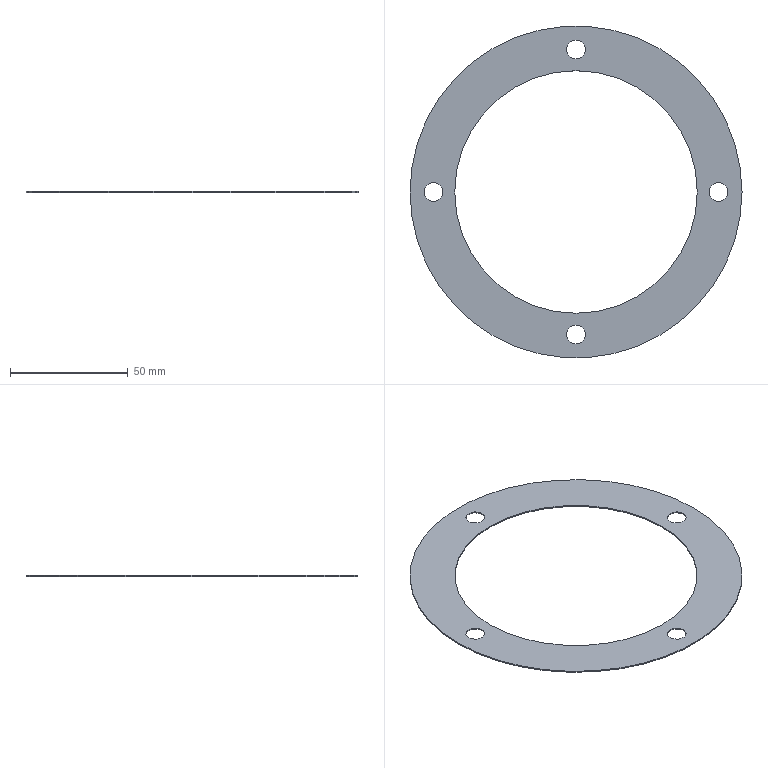Part | SolidWorks | features Extrusion 1, ICE 1 | 1 solid | 14 faces | box 141 x 141 x 0.5 mm | volume 3541 mm3 | cylinder 12 | plane 2 | commonest cylinder face diameters 8 x8 103 x2 141 x2
STEP:
#1=CARTESIAN_POINT('',(-64.5,0.,0.));
#2=VERTEX_POINT('',#1);
#3=CARTESIAN_POINT('',(-56.5,0.,0.));
#4=VERTEX_POINT('',#3);
#5=CARTESIAN_POINT('',(-60.5,0.,0.));
#6=DIRECTION('',(0.,0.,1.));
#7=DIRECTION('',(1.,0.,0.));
#8=AXIS2_PLACEMENT_3D('',#5,#6,#7);
#9=CIRCLE('',#8,4.);
#10=EDGE_CURVE('',#2,#4,#9,.T.);
#11=ORIENTED_EDGE('',*,*,#10,.F.);
#12=CARTESIAN_POINT('',(-64.5,0.,0.5));
#13=VERTEX_POINT('',#12);
#14=CARTESIAN_POINT('',(-64.5,0.,0.));
#15=DIRECTION('',(0.,0.,1.));
#16=VECTOR('',#15,1000.);
#17=LINE('',#14,#16);
#18=EDGE_CURVE('',#2,#13,#17,.T.);
#19=ORIENTED_EDGE('',*,*,#18,.T.);
#20=CARTESIAN_POINT('',(-56.5,0.,0.5));
#21=VERTEX_POINT('',#20);
#22=CARTESIAN_POINT('',(-60.5,0.,0.5));
#23=DIRECTION('',(0.,0.,1.));
#24=DIRECTION('',(1.,0.,0.));
#25=AXIS2_PLACEMENT_3D('',#22,#23,#24);
#26=CIRCLE('',#25,4.);
#27=EDGE_CURVE('',#13,#21,#26,.T.);
#28=ORIENTED_EDGE('',*,*,#27,.T.);
#29=CARTESIAN_POINT('',(-56.5,0.,0.));
#30=DIRECTION('',(0.,0.,1.));
#31=VECTOR('',#30,1000.);
#32=LINE('',#29,#31);
#33=EDGE_CURVE('',#4,#21,#32,.T.);
#34=ORIENTED_EDGE('',*,*,#33,.F.);
#35=EDGE_LOOP('',(#11,#19,#28,#34));
#36=FACE_OUTER_BOUND('',#35,.T.);
#37=CARTESIAN_POINT('',(-60.5,0.,0.));
#38=DIRECTION('',(0.,0.,1.));
#39=DIRECTION('',(1.,0.,0.));
#40=AXIS2_PLACEMENT_3D('',#37,#38,#39);
#41=CYLINDRICAL_SURFACE('',#40,4.);
#42=ADVANCED_FACE('',(#36),#41,.F.);
#43=CARTESIAN_POINT('',(-4.,60.5,0.));
#44=VERTEX_POINT('',#43);
#45=CARTESIAN_POINT('',(4.,60.5,0.));
#46=VERTEX_POINT('',#45);
#47=CARTESIAN_POINT('',(0.,60.5,0.));
#48=DIRECTION('',(0.,0.,1.));
#49=DIRECTION('',(1.,0.,0.));
#50=AXIS2_PLACEMENT_3D('',#47,#48,#49);
#51=CIRCLE('',#50,4.);
#52=EDGE_CURVE('',#44,#46,#51,.T.);
#53=ORIENTED_EDGE('',*,*,#52,.F.);
#54=CARTESIAN_POINT('',(-4.,60.5,0.5));
#55=VERTEX_POINT('',#54);
#56=CARTESIAN_POINT('',(-4.,60.5,0.));
#57=DIRECTION('',(0.,0.,1.));
#58=VECTOR('',#57,1000.);
#59=LINE('',#56,#58);
#60=EDGE_CURVE('',#44,#55,#59,.T.);
#61=ORIENTED_EDGE('',*,*,#60,.T.);
#62=CARTESIAN_POINT('',(4.,60.5,0.5));
#63=VERTEX_POINT('',#62);
#64=CARTESIAN_POINT('',(0.,60.5,0.5));
#65=DIRECTION('',(0.,0.,1.));
#66=DIRECTION('',(1.,0.,0.));
#67=AXIS2_PLACEMENT_3D('',#64,#65,#66);
#68=CIRCLE('',#67,4.);
#69=EDGE_CURVE('',#55,#63,#68,.T.);
#70=ORIENTED_EDGE('',*,*,#69,.T.);
#71=CARTESIAN_POINT('',(4.,60.5,0.));
#72=DIRECTION('',(0.,0.,1.));
#73=VECTOR('',#72,1000.);
#74=LINE('',#71,#73);
#75=EDGE_CURVE('',#46,#63,#74,.T.);
#76=ORIENTED_EDGE('',*,*,#75,.F.);
#77=EDGE_LOOP('',(#53,#61,#70,#76));
#78=FACE_OUTER_BOUND('',#77,.T.);
#79=CARTESIAN_POINT('',(0.,60.5,0.));
#80=DIRECTION('',(0.,0.,1.));
#81=DIRECTION('',(1.,0.,0.));
#82=AXIS2_PLACEMENT_3D('',#79,#80,#81);
#83=CYLINDRICAL_SURFACE('',#82,4.);
#84=ADVANCED_FACE('',(#78),#83,.F.);
#85=CARTESIAN_POINT('',(56.5,0.,0.));
#86=VERTEX_POINT('',#85);
#87=CARTESIAN_POINT('',(64.5,0.,0.));
#88=VERTEX_POINT('',#87);
#89=CARTESIAN_POINT('',(60.5,0.,0.));
#90=DIRECTION('',(0.,0.,1.));
#91=DIRECTION('',(1.,0.,0.));
#92=AXIS2_PLACEMENT_3D('',#89,#90,#91);
#93=CIRCLE('',#92,4.);
#94=EDGE_CURVE('',#86,#88,#93,.T.);
#95=ORIENTED_EDGE('',*,*,#94,.F.);
#96=CARTESIAN_POINT('',(56.5,0.,0.5));
#97=VERTEX_POINT('',#96);
#98=CARTESIAN_POINT('',(56.5,0.,0.));
#99=DIRECTION('',(0.,0.,1.));
#100=VECTOR('',#99,1000.);
#101=LINE('',#98,#100);
#102=EDGE_CURVE('',#86,#97,#101,.T.);
#103=ORIENTED_EDGE('',*,*,#102,.T.);
#104=CARTESIAN_POINT('',(64.5,0.,0.5));
#105=VERTEX_POINT('',#104);
#106=CARTESIAN_POINT('',(60.5,0.,0.5));
#107=DIRECTION('',(0.,0.,1.));
#108=DIRECTION('',(1.,0.,0.));
#109=AXIS2_PLACEMENT_3D('',#106,#107,#108);
#110=CIRCLE('',#109,4.);
#111=EDGE_CURVE('',#97,#105,#110,.T.);
#112=ORIENTED_EDGE('',*,*,#111,.T.);
#113=CARTESIAN_POINT('',(64.5,0.,0.));
#114=DIRECTION('',(0.,0.,1.));
#115=VECTOR('',#114,1000.);
#116=LINE('',#113,#115);
#117=EDGE_CURVE('',#88,#105,#116,.T.);
#118=ORIENTED_EDGE('',*,*,#117,.F.);
#119=EDGE_LOOP('',(#95,#103,#112,#118));
#120=FACE_OUTER_BOUND('',#119,.T.);
#121=CARTESIAN_POINT('',(60.5,0.,0.));
#122=DIRECTION('',(0.,0.,1.));
#123=DIRECTION('',(1.,0.,0.));
#124=AXIS2_PLACEMENT_3D('',#121,#122,#123);
#125=CYLINDRICAL_SURFACE('',#124,4.);
#126=ADVANCED_FACE('',(#120),#125,.F.);
#127=CARTESIAN_POINT('',(-4.,-60.5,0.));
#128=VERTEX_POINT('',#127);
#129=CARTESIAN_POINT('',(4.,-60.5,0.));
#130=VERTEX_POINT('',#129);
#131=CARTESIAN_POINT('',(0.,-60.5,0.));
#132=DIRECTION('',(0.,0.,1.));
#133=DIRECTION('',(1.,0.,0.));
#134=AXIS2_PLACEMENT_3D('',#131,#132,#133);
#135=CIRCLE('',#134,4.);
#136=EDGE_CURVE('',#128,#130,#135,.T.);
#137=ORIENTED_EDGE('',*,*,#136,.F.);
#138=CARTESIAN_POINT('',(-4.,-60.5,0.5));
#139=VERTEX_POINT('',#138);
#140=CARTESIAN_POINT('',(-4.,-60.5,0.));
#141=DIRECTION('',(0.,0.,1.));
#142=VECTOR('',#141,1000.);
#143=LINE('',#140,#142);
#144=EDGE_CURVE('',#128,#139,#143,.T.);
#145=ORIENTED_EDGE('',*,*,#144,.T.);
#146=CARTESIAN_POINT('',(4.,-60.5,0.5));
#147=VERTEX_POINT('',#146);
#148=CARTESIAN_POINT('',(0.,-60.5,0.5));
#149=DIRECTION('',(0.,0.,1.));
#150=DIRECTION('',(1.,0.,0.));
#151=AXIS2_PLACEMENT_3D('',#148,#149,#150);
#152=CIRCLE('',#151,4.);
#153=EDGE_CURVE('',#139,#147,#152,.T.);
#154=ORIENTED_EDGE('',*,*,#153,.T.);
#155=CARTESIAN_POINT('',(4.,-60.5,0.));
#156=DIRECTION('',(0.,0.,1.));
#157=VECTOR('',#156,1000.);
#158=LINE('',#155,#157);
#159=EDGE_CURVE('',#130,#147,#158,.T.);
#160=ORIENTED_EDGE('',*,*,#159,.F.);
#161=EDGE_LOOP('',(#137,#145,#154,#160));
#162=FACE_OUTER_BOUND('',#161,.T.);
#163=CARTESIAN_POINT('',(0.,-60.5,0.));
#164=DIRECTION('',(0.,0.,1.));
#165=DIRECTION('',(1.,0.,0.));
#166=AXIS2_PLACEMENT_3D('',#163,#164,#165);
#167=CYLINDRICAL_SURFACE('',#166,4.);
#168=ADVANCED_FACE('',(#162),#167,.F.);
#169=CARTESIAN_POINT('',(-51.5,0.,0.5));
#170=VERTEX_POINT('',#169);
#171=CARTESIAN_POINT('',(51.5,0.,0.5));
#172=VERTEX_POINT('',#171);
#173=CARTESIAN_POINT('',(0.,0.,0.5));
#174=DIRECTION('',(0.,0.,1.));
#175=DIRECTION('',(1.,0.,0.));
#176=AXIS2_PLACEMENT_3D('',#173,#174,#175);
#177=CIRCLE('',#176,51.5);
#178=EDGE_CURVE('',#170,#172,#177,.T.);
#179=ORIENTED_EDGE('',*,*,#178,.T.);
#180=CARTESIAN_POINT('',(51.5,0.,0.));
#181=VERTEX_POINT('',#180);
#182=CARTESIAN_POINT('',(51.5,0.,0.5));
#183=DIRECTION('',(0.,0.,-1.));
#184=VECTOR('',#183,1000.);
#185=LINE('',#182,#184);
#186=EDGE_CURVE('',#172,#181,#185,.T.);
#187=ORIENTED_EDGE('',*,*,#186,.T.);
#188=CARTESIAN_POINT('',(-51.5,0.,0.));
#189=VERTEX_POINT('',#188);
#190=CARTESIAN_POINT('',(0.,0.,0.));
#191=DIRECTION('',(0.,0.,1.));
#192=DIRECTION('',(1.,0.,0.));
#193=AXIS2_PLACEMENT_3D('',#190,#191,#192);
#194=CIRCLE('',#193,51.5);
#195=EDGE_CURVE('',#189,#181,#194,.T.);
#196=ORIENTED_EDGE('',*,*,#195,.F.);
#197=CARTESIAN_POINT('',(-51.5,0.,0.5));
#198=DIRECTION('',(0.,0.,-1.));
#199=VECTOR('',#198,1000.);
#200=LINE('',#197,#199);
#201=EDGE_CURVE('',#170,#189,#200,.T.);
#202=ORIENTED_EDGE('',*,*,#201,.F.);
#203=EDGE_LOOP('',(#179,#187,#196,#202));
#204=FACE_OUTER_BOUND('',#203,.T.);
#205=CARTESIAN_POINT('',(0.,0.,0.5));
#206=DIRECTION('',(0.,0.,-1.));
#207=DIRECTION('',(-1.,0.,0.));
#208=AXIS2_PLACEMENT_3D('',#205,#206,#207);
#209=CYLINDRICAL_SURFACE('',#208,51.5);
#210=ADVANCED_FACE('',(#204),#209,.F.);
#211=CARTESIAN_POINT('',(70.5,0.,0.5));
#212=VERTEX_POINT('',#211);
#213=CARTESIAN_POINT('',(-70.5,0.,0.5));
#214=VERTEX_POINT('',#213);
#215=CARTESIAN_POINT('',(0.,0.,0.5));
#216=DIRECTION('',(0.,0.,1.));
#217=DIRECTION('',(1.,0.,0.));
#218=AXIS2_PLACEMENT_3D('',#215,#216,#217);
#219=CIRCLE('',#218,70.5);
#220=EDGE_CURVE('',#212,#214,#219,.T.);
#221=ORIENTED_EDGE('',*,*,#220,.F.);
#222=CARTESIAN_POINT('',(70.5,0.,0.));
#223=VERTEX_POINT('',#222);
#224=CARTESIAN_POINT('',(70.5,0.,0.5));
#225=DIRECTION('',(0.,0.,-1.));
#226=VECTOR('',#225,1000.);
#227=LINE('',#224,#226);
#228=EDGE_CURVE('',#212,#223,#227,.T.);
#229=ORIENTED_EDGE('',*,*,#228,.T.);
#230=CARTESIAN_POINT('',(-70.5,0.,0.));
#231=VERTEX_POINT('',#230);
#232=CARTESIAN_POINT('',(0.,0.,0.));
#233=DIRECTION('',(0.,0.,1.));
#234=DIRECTION('',(1.,0.,0.));
#235=AXIS2_PLACEMENT_3D('',#232,#233,#234);
#236=CIRCLE('',#235,70.5);
#237=EDGE_CURVE('',#223,#231,#236,.T.);
#238=ORIENTED_EDGE('',*,*,#237,.T.);
#239=CARTESIAN_POINT('',(-70.5,0.,0.5));
#240=DIRECTION('',(0.,0.,-1.));
#241=VECTOR('',#240,1000.);
#242=LINE('',#239,#241);
#243=EDGE_CURVE('',#214,#231,#242,.T.);
#244=ORIENTED_EDGE('',*,*,#243,.F.);
#245=EDGE_LOOP('',(#221,#229,#238,#244));
#246=FACE_OUTER_BOUND('',#245,.T.);
#247=CARTESIAN_POINT('',(0.,0.,0.5));
#248=DIRECTION('',(0.,0.,-1.));
#249=DIRECTION('',(-1.,0.,0.));
#250=AXIS2_PLACEMENT_3D('',#247,#248,#249);
#251=CYLINDRICAL_SURFACE('',#250,70.5);
#252=ADVANCED_FACE('',(#246),#251,.T.);
#253=CARTESIAN_POINT('',(-60.5,0.,0.5));
#254=DIRECTION('',(0.,0.,1.));
#255=DIRECTION('',(1.,0.,0.));
#256=AXIS2_PLACEMENT_3D('',#253,#254,#255);
#257=CIRCLE('',#256,4.);
#258=EDGE_CURVE('',#21,#13,#257,.T.);
#259=ORIENTED_EDGE('',*,*,#258,.F.);
#260=ORIENTED_EDGE('',*,*,#27,.F.);
#261=EDGE_LOOP('',(#259,#260));
#262=FACE_BOUND('',#261,.T.);
#263=CARTESIAN_POINT('',(0.,60.5,0.5));
#264=DIRECTION('',(0.,0.,1.));
#265=DIRECTION('',(1.,0.,0.));
#266=AXIS2_PLACEMENT_3D('',#263,#264,#265);
#267=CIRCLE('',#266,4.);
#268=EDGE_CURVE('',#63,#55,#267,.T.);
#269=ORIENTED_EDGE('',*,*,#268,.F.);
#270=ORIENTED_EDGE('',*,*,#69,.F.);
#271=EDGE_LOOP('',(#269,#270));
#272=FACE_BOUND('',#271,.T.);
#273=CARTESIAN_POINT('',(60.5,0.,0.5));
#274=DIRECTION('',(0.,0.,1.));
#275=DIRECTION('',(1.,0.,0.));
#276=AXIS2_PLACEMENT_3D('',#273,#274,#275);
#277=CIRCLE('',#276,4.);
#278=EDGE_CURVE('',#105,#97,#277,.T.);
#279=ORIENTED_EDGE('',*,*,#278,.F.);
#280=ORIENTED_EDGE('',*,*,#111,.F.);
#281=EDGE_LOOP('',(#279,#280));
#282=FACE_BOUND('',#281,.T.);
#283=CARTESIAN_POINT('',(0.,-60.5,0.5));
#284=DIRECTION('',(0.,0.,1.));
#285=DIRECTION('',(1.,0.,0.));
#286=AXIS2_PLACEMENT_3D('',#283,#284,#285);
#287=CIRCLE('',#286,4.);
#288=EDGE_CURVE('',#147,#139,#287,.T.);
#289=ORIENTED_EDGE('',*,*,#288,.F.);
#290=ORIENTED_EDGE('',*,*,#153,.F.);
#291=EDGE_LOOP('',(#289,#290));
#292=FACE_BOUND('',#291,.T.);
#293=CARTESIAN_POINT('',(0.,0.,0.5));
#294=DIRECTION('',(0.,0.,1.));
#295=DIRECTION('',(1.,0.,0.));
#296=AXIS2_PLACEMENT_3D('',#293,#294,#295);
#297=CIRCLE('',#296,70.5);
#298=EDGE_CURVE('',#214,#212,#297,.T.);
#299=ORIENTED_EDGE('',*,*,#298,.T.);
#300=ORIENTED_EDGE('',*,*,#220,.T.);
#301=EDGE_LOOP('',(#299,#300));
#302=FACE_OUTER_BOUND('',#301,.T.);
#303=ORIENTED_EDGE('',*,*,#178,.F.);
#304=CARTESIAN_POINT('',(0.,0.,0.5));
#305=DIRECTION('',(0.,0.,1.));
#306=DIRECTION('',(1.,0.,0.));
#307=AXIS2_PLACEMENT_3D('',#304,#305,#306);
#308=CIRCLE('',#307,51.5);
#309=EDGE_CURVE('',#172,#170,#308,.T.);
#310=ORIENTED_EDGE('',*,*,#309,.F.);
#311=EDGE_LOOP('',(#303,#310));
#312=FACE_BOUND('',#311,.T.);
#313=CARTESIAN_POINT('',(0.,0.,0.5));
#314=DIRECTION('',(0.,0.,1.));
#315=DIRECTION('',(1.,0.,0.));
#316=AXIS2_PLACEMENT_3D('',#313,#314,#315);
#317=PLANE('',#316);
#318=ADVANCED_FACE('',(#262,#272,#282,#292,#302,#312),#317,.T.);
#319=CARTESIAN_POINT('',(-60.5,0.,0.));
#320=DIRECTION('',(0.,0.,1.));
#321=DIRECTION('',(1.,0.,0.));
#322=AXIS2_PLACEMENT_3D('',#319,#320,#321);
#323=CIRCLE('',#322,4.);
#324=EDGE_CURVE('',#4,#2,#323,.T.);
#325=ORIENTED_EDGE('',*,*,#324,.T.);
#326=ORIENTED_EDGE('',*,*,#10,.T.);
#327=EDGE_LOOP('',(#325,#326));
#328=FACE_BOUND('',#327,.T.);
#329=CARTESIAN_POINT('',(0.,60.5,0.));
#330=DIRECTION('',(0.,0.,1.));
#331=DIRECTION('',(1.,0.,0.));
#332=AXIS2_PLACEMENT_3D('',#329,#330,#331);
#333=CIRCLE('',#332,4.);
#334=EDGE_CURVE('',#46,#44,#333,.T.);
#335=ORIENTED_EDGE('',*,*,#334,.T.);
#336=ORIENTED_EDGE('',*,*,#52,.T.);
#337=EDGE_LOOP('',(#335,#336));
#338=FACE_BOUND('',#337,.T.);
#339=CARTESIAN_POINT('',(60.5,0.,0.));
#340=DIRECTION('',(0.,0.,1.));
#341=DIRECTION('',(1.,0.,0.));
#342=AXIS2_PLACEMENT_3D('',#339,#340,#341);
#343=CIRCLE('',#342,4.);
#344=EDGE_CURVE('',#88,#86,#343,.T.);
#345=ORIENTED_EDGE('',*,*,#344,.T.);
#346=ORIENTED_EDGE('',*,*,#94,.T.);
#347=EDGE_LOOP('',(#345,#346));
#348=FACE_BOUND('',#347,.T.);
#349=CARTESIAN_POINT('',(0.,-60.5,0.));
#350=DIRECTION('',(0.,0.,1.));
#351=DIRECTION('',(1.,0.,0.));
#352=AXIS2_PLACEMENT_3D('',#349,#350,#351);
#353=CIRCLE('',#352,4.);
#354=EDGE_CURVE('',#130,#128,#353,.T.);
#355=ORIENTED_EDGE('',*,*,#354,.T.);
#356=ORIENTED_EDGE('',*,*,#136,.T.);
#357=EDGE_LOOP('',(#355,#356));
#358=FACE_BOUND('',#357,.T.);
#359=CARTESIAN_POINT('',(0.,0.,0.));
#360=DIRECTION('',(0.,0.,1.));
#361=DIRECTION('',(1.,0.,0.));
#362=AXIS2_PLACEMENT_3D('',#359,#360,#361);
#363=CIRCLE('',#362,70.5);
#364=EDGE_CURVE('',#231,#223,#363,.T.);
#365=ORIENTED_EDGE('',*,*,#364,.F.);
#366=ORIENTED_EDGE('',*,*,#237,.F.);
#367=EDGE_LOOP('',(#365,#366));
#368=FACE_OUTER_BOUND('',#367,.T.);
#369=ORIENTED_EDGE('',*,*,#195,.T.);
#370=CARTESIAN_POINT('',(0.,0.,0.));
#371=DIRECTION('',(0.,0.,1.));
#372=DIRECTION('',(1.,0.,0.));
#373=AXIS2_PLACEMENT_3D('',#370,#371,#372);
#374=CIRCLE('',#373,51.5);
#375=EDGE_CURVE('',#181,#189,#374,.T.);
#376=ORIENTED_EDGE('',*,*,#375,.T.);
#377=EDGE_LOOP('',(#369,#376));
#378=FACE_BOUND('',#377,.T.);
#379=CARTESIAN_POINT('',(0.,0.,0.));
#380=DIRECTION('',(0.,0.,1.));
#381=DIRECTION('',(1.,0.,0.));
#382=AXIS2_PLACEMENT_3D('',#379,#380,#381);
#383=PLANE('',#382);
#384=ADVANCED_FACE('',(#328,#338,#348,#358,#368,#378),#383,.F.);
#385=ORIENTED_EDGE('',*,*,#228,.F.);
#386=ORIENTED_EDGE('',*,*,#298,.F.);
#387=ORIENTED_EDGE('',*,*,#243,.T.);
#388=ORIENTED_EDGE('',*,*,#364,.T.);
#389=EDGE_LOOP('',(#385,#386,#387,#388));
#390=FACE_OUTER_BOUND('',#389,.T.);
#391=CARTESIAN_POINT('',(0.,0.,0.5));
#392=DIRECTION('',(0.,0.,-1.));
#393=DIRECTION('',(-1.,0.,0.));
#394=AXIS2_PLACEMENT_3D('',#391,#392,#393);
#395=CYLINDRICAL_SURFACE('',#394,70.5);
#396=ADVANCED_FACE('',(#390),#395,.T.);
#397=ORIENTED_EDGE('',*,*,#186,.F.);
#398=ORIENTED_EDGE('',*,*,#309,.T.);
#399=ORIENTED_EDGE('',*,*,#201,.T.);
#400=ORIENTED_EDGE('',*,*,#375,.F.);
#401=EDGE_LOOP('',(#397,#398,#399,#400));
#402=FACE_OUTER_BOUND('',#401,.T.);
#403=CARTESIAN_POINT('',(0.,0.,0.5));
#404=DIRECTION('',(0.,0.,-1.));
#405=DIRECTION('',(-1.,0.,0.));
#406=AXIS2_PLACEMENT_3D('',#403,#404,#405);
#407=CYLINDRICAL_SURFACE('',#406,51.5);
#408=ADVANCED_FACE('',(#402),#407,.F.);
#409=ORIENTED_EDGE('',*,*,#144,.F.);
#410=ORIENTED_EDGE('',*,*,#354,.F.);
#411=ORIENTED_EDGE('',*,*,#159,.T.);
#412=ORIENTED_EDGE('',*,*,#288,.T.);
#413=EDGE_LOOP('',(#409,#410,#411,#412));
#414=FACE_OUTER_BOUND('',#413,.T.);
#415=CARTESIAN_POINT('',(0.,-60.5,0.));
#416=DIRECTION('',(0.,0.,1.));
#417=DIRECTION('',(1.,0.,0.));
#418=AXIS2_PLACEMENT_3D('',#415,#416,#417);
#419=CYLINDRICAL_SURFACE('',#418,4.);
#420=ADVANCED_FACE('',(#414),#419,.F.);
#421=ORIENTED_EDGE('',*,*,#102,.F.);
#422=ORIENTED_EDGE('',*,*,#344,.F.);
#423=ORIENTED_EDGE('',*,*,#117,.T.);
#424=ORIENTED_EDGE('',*,*,#278,.T.);
#425=EDGE_LOOP('',(#421,#422,#423,#424));
#426=FACE_OUTER_BOUND('',#425,.T.);
#427=CARTESIAN_POINT('',(60.5,0.,0.));
#428=DIRECTION('',(0.,0.,1.));
#429=DIRECTION('',(1.,0.,0.));
#430=AXIS2_PLACEMENT_3D('',#427,#428,#429);
#431=CYLINDRICAL_SURFACE('',#430,4.);
#432=ADVANCED_FACE('',(#426),#431,.F.);
#433=ORIENTED_EDGE('',*,*,#60,.F.);
#434=ORIENTED_EDGE('',*,*,#334,.F.);
#435=ORIENTED_EDGE('',*,*,#75,.T.);
#436=ORIENTED_EDGE('',*,*,#268,.T.);
#437=EDGE_LOOP('',(#433,#434,#435,#436));
#438=FACE_OUTER_BOUND('',#437,.T.);
#439=CARTESIAN_POINT('',(0.,60.5,0.));
#440=DIRECTION('',(0.,0.,1.));
#441=DIRECTION('',(1.,0.,0.));
#442=AXIS2_PLACEMENT_3D('',#439,#440,#441);
#443=CYLINDRICAL_SURFACE('',#442,4.);
#444=ADVANCED_FACE('',(#438),#443,.F.);
#445=ORIENTED_EDGE('',*,*,#18,.F.);
#446=ORIENTED_EDGE('',*,*,#324,.F.);
#447=ORIENTED_EDGE('',*,*,#33,.T.);
#448=ORIENTED_EDGE('',*,*,#258,.T.);
#449=EDGE_LOOP('',(#445,#446,#447,#448));
#450=FACE_OUTER_BOUND('',#449,.T.);
#451=CARTESIAN_POINT('',(-60.5,0.,0.));
#452=DIRECTION('',(0.,0.,1.));
#453=DIRECTION('',(1.,0.,0.));
#454=AXIS2_PLACEMENT_3D('',#451,#452,#453);
#455=CYLINDRICAL_SURFACE('',#454,4.);
#456=ADVANCED_FACE('',(#450),#455,.F.);
#457=CLOSED_SHELL('',(#42,#84,#126,#168,#210,#252,#318,#384,#396,#408,#420,#432,#444,#456));
#458=MANIFOLD_SOLID_BREP('',#457);
#459=CARTESIAN_POINT('',(0.,0.,0.));
#460=DIRECTION('',(0.,0.,1.));
#461=DIRECTION('',(1.,0.,0.));
#462=AXIS2_PLACEMENT_3D('',#459,#460,#461);
#463=(LENGTH_UNIT()NAMED_UNIT(*)SI_UNIT(.MILLI.,.METRE.));
#464=UNCERTAINTY_MEASURE_WITH_UNIT(LENGTH_MEASURE(0.00001),#463,'','');
#465=(NAMED_UNIT(*)PLANE_ANGLE_UNIT()SI_UNIT($,.RADIAN.));
#466=(NAMED_UNIT(*)SI_UNIT($,.STERADIAN.)SOLID_ANGLE_UNIT());
#467=(GEOMETRIC_REPRESENTATION_CONTEXT(3)GLOBAL_UNCERTAINTY_ASSIGNED_CONTEXT((#464))GLOBAL_UNIT_ASSIGNED_CONTEXT((#463,#465,#466))REPRESENTATION_CONTEXT('',''));
#468=ADVANCED_BREP_SHAPE_REPRESENTATION('',(#458,#462),#467);